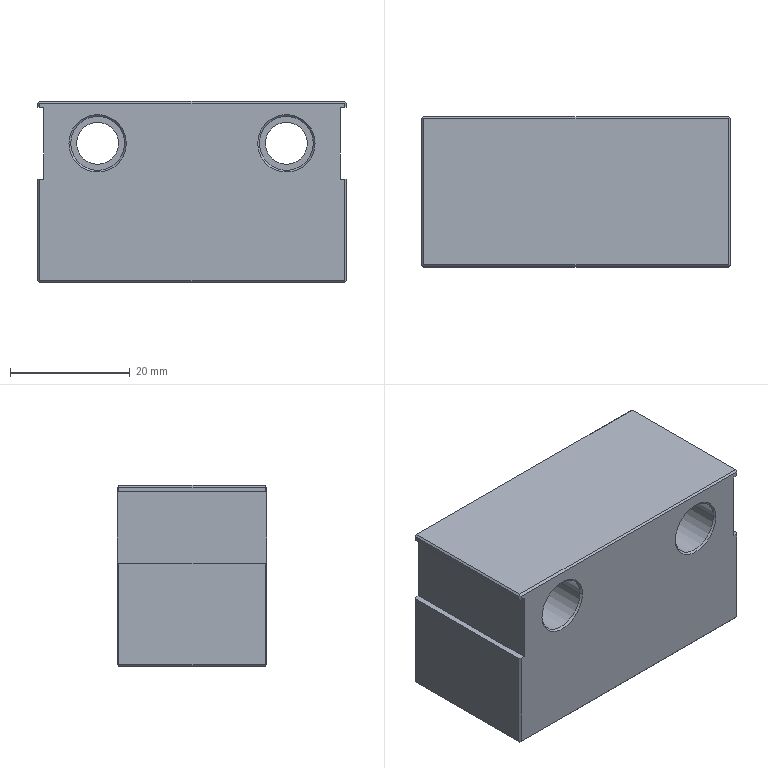Part | NX | 1 solid | 78 faces | box 51.5 x 25 x 30.237 mm | volume 34829 mm3 | plane 34 | cylinder 24 | cone 20 | commonest cylinder face diameters 3.3 x8 9 x8 4 x4 7 x4